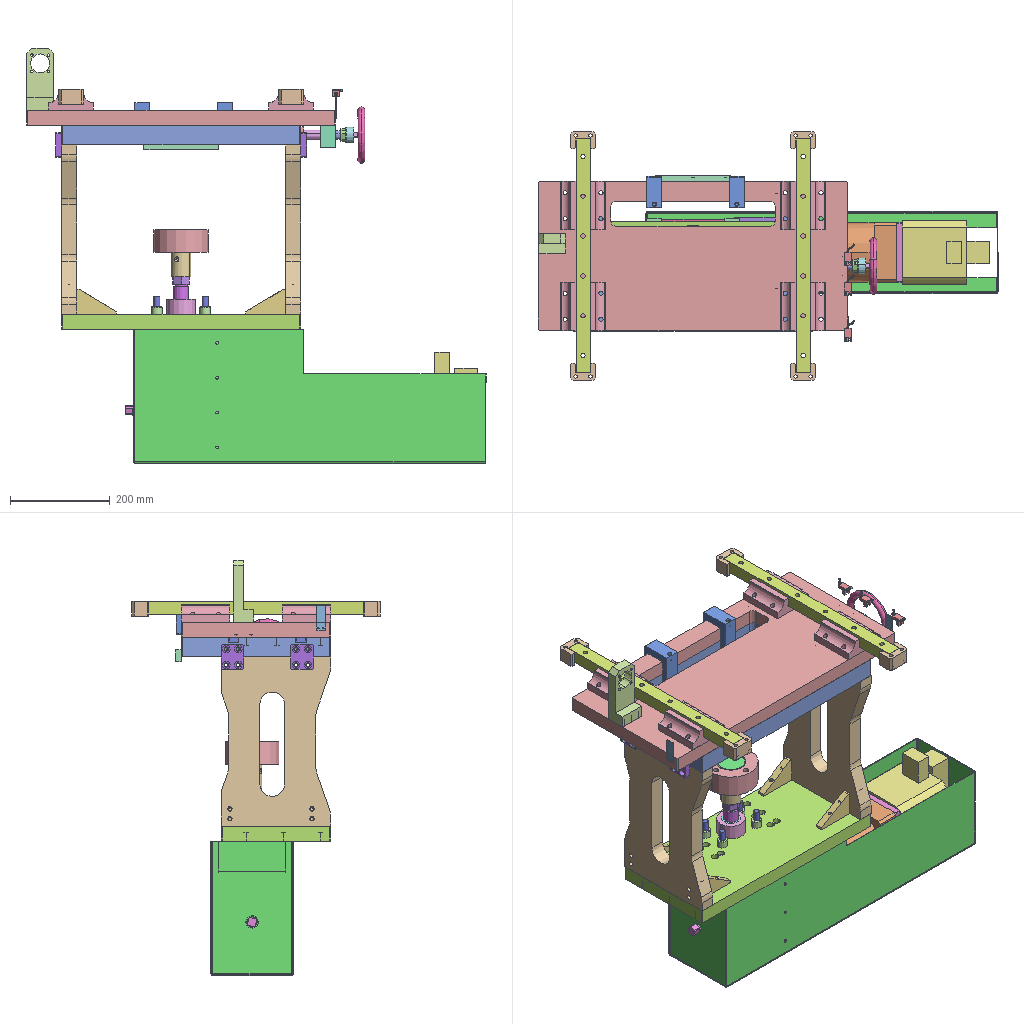Assembly | SolidWorks | 53 different items | 86 placed | box 924 x 500 x 834 mm
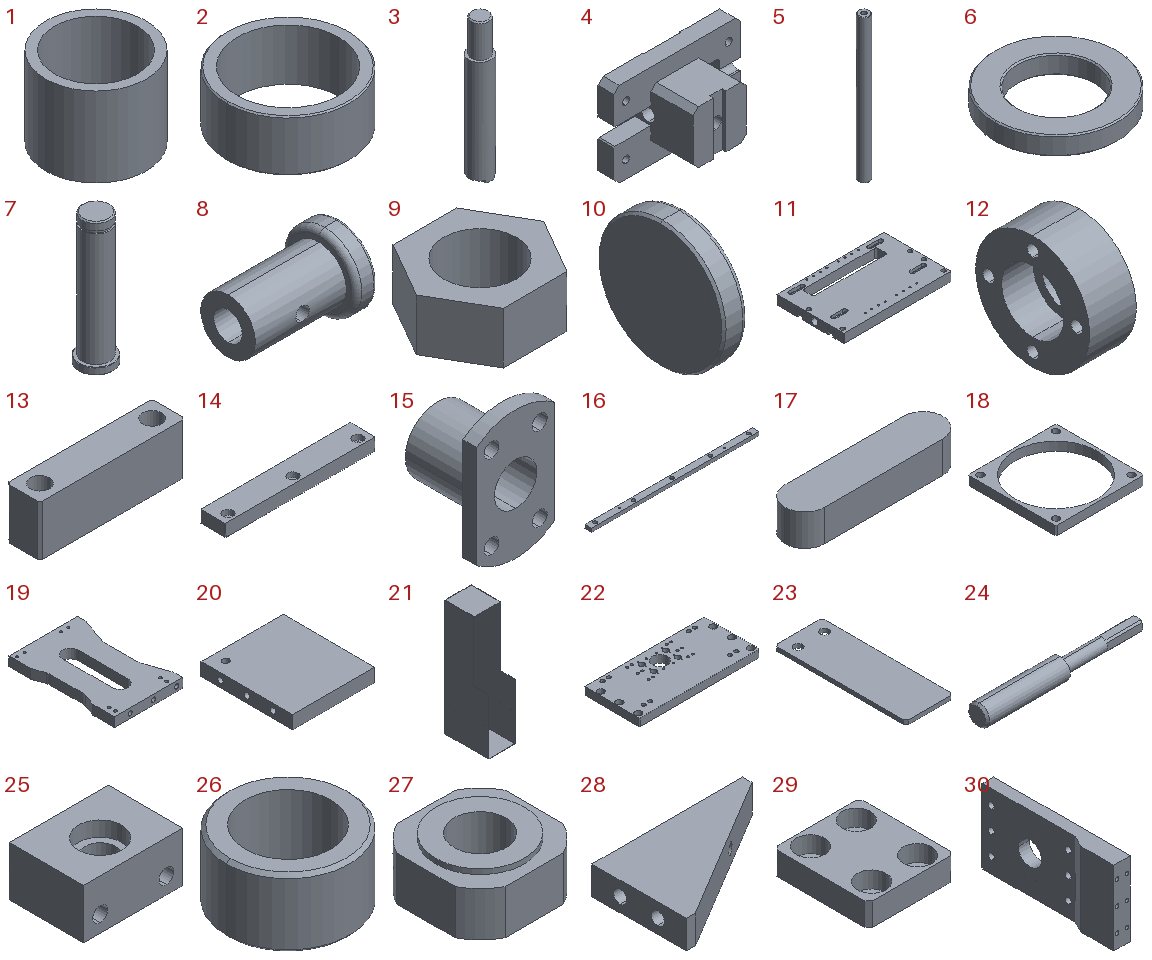Parts list (item | quantity | size | volume | features):
1 | x1 | 48 x 48 x 38 mm | 22197 mm3 | features Extrusion 1
2 | x1 | 48 x 48 x 20 mm | 11645 mm3 | features Chamfer 1, Extrusion 1
3 | x1 | 30 x 30 x 188 mm | 118848 mm3 | features ICE 2, Chamfer 1, Extrusion 1, HoleWzd 1
4 | x1 | 120 x 55 x 80 mm | 190025 mm3 | features ICE 7, Chamfer 2, HoleWzd 2, Extrusion 1
5 | x4 | 12 x 12 x 160 mm | 17782 mm3 | features Chamfer 1, Extrusion 1, HoleWzd 1
6 | x4 | 20 x 20 x 3 mm | 570.238 mm3 | features Chamfer 1, Extrusion 1
7 | x1 | 15 x 15 x 57.5 mm | 6667 mm3 | features Chamfer 2, Extrusion 1, ICE 1, RefAxis 1, RevCut 1
8 | x1 | 82 x 55 x 55 mm | 93090 mm3 | features Fillet 2, HoleWzd 1, ICE 1, Revolution 1
9 | x1 | 36.95 x 32 x 15 mm | 8107 mm3 | features Extrusion 1, HoleWzd 1
10 | x1 | 16.494 x 58 x 58 mm | 35001 mm3 | features Chamfer 1, Fillet 1, Revolution 1
11 | x1 | 480 x 300 x 40 mm | 4575691 mm3 | features HoleWzd 6, ICE 6, Chamfer 1, Extrusion 1, MirrorPattern 1
12 | x1 | 45 x 110 x 110 mm | 290495 mm3 | features HoleWzd 1, Revolution 1
13 | x1 | 26 x 6 x 9 mm | 1236 mm3 | features Chamfer 1, Extrusion 1, HoleWzd 1
14 | x1 | 150 x 25 x 12 mm | 43317 mm3 | features Chamfer 1, Extrusion 1, HoleWzd 1
15 | x1 | 34 x 34 x 56 mm | 17982 mm3 | features HoleWzd 2, ICE 1, Revolution 1
16 | x2 | 480 x 20 x 10 mm | 92979 mm3 | features HoleWzd 2, Chamfer 1, Extrusion 1
17 | x1 | 40 x 10 x 8 mm | 3028 mm3 | features Extrusion 1
18 | x1 | 120 x 120 x 12 mm | 51426 mm3 | features Chamfer 1, CirPattern 1, Extrusion 1, HoleWzd 1, ICE 1
19 | x2 | 220 x 340 x 30 mm | 1630627 mm3 | features HoleWzd 4, Cut 1, Extrusion 1
20 | x2 | 125 x 140 x 20 mm | 339828 mm3 | features HoleWzd 2, Extrusion 1, ICE 1
21 | x1 | 165 x 270 x 708 mm | 725999 mm3 | features EdgeFlange 2, ICE 2, Cut 1, FlatPattern 1, SMBaseFlange 1, SheetMetal 1
22 | x1 | 480 x 220 x 30 mm | 2905739 mm3 | features HoleWzd 5, Chamfer 1, Cut 1, Extrusion 1, ICE 1, MirrorPattern 1
23 | x2 | 18 x 50 x 1.5 mm | 1323 mm3 | features Chamfer 1, Extrusion 1, HoleWzd 1
24 | x1 | 155 x 20 x 20 mm | 32861 mm3 | features Chamfer 2, ICE 1, Revolution 1
25 | x1 | 60 x 45 x 30 mm | 60481 mm3 | features ICE 2, Extrusion 1, HoleWzd 1
26 | x1 | 18 x 18 x 10 mm | 1304 mm3 | features Chamfer 1, Extrusion 1
27 | x1 | 22 x 22 x 10 mm | 3311 mm3 | features HoleWzd 2, 3DProfileFeature 1, Extrusion 1, ICE 1
28 | x4 | 80 x 50 x 15 mm | 31407 mm3 | features HoleWzd 2, Extrusion 1
29 | x4 | 45 x 50 x 12 mm | 19960 mm3 | features Chamfer 1, Extrusion 1, HoleWzd 1
30 | x2 | 30 x 250 x 135 mm | 713772 mm3 | features HoleWzd 4, Chamfer 1, Extrusion 1, ICE 1
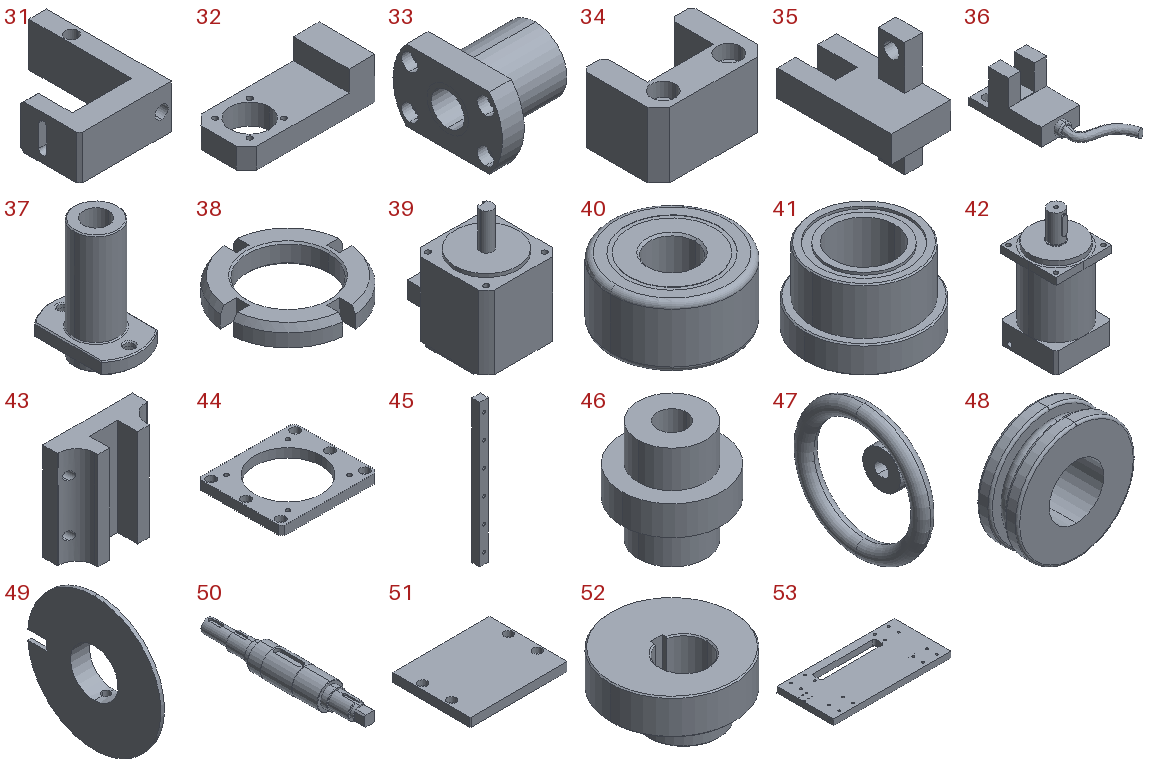31 | x2 | 62.5 x 85 x 30 mm | 56190 mm3 | features ICE 4, HoleWzd 2, Chamfer 1, Extrusion 1
32 | x1 | 124 x 54 x 40 mm | 132841 mm3 | features HoleWzd 2, ICE 2, Chamfer 1, CirPattern 1, Extrusion 1
33 | x1 | 80 x 100 x 65 mm | 212969 mm3 | features ICE 3, HoleWzd 1, Revolution 1
34 | x4 | 50 x 35 x 30 mm | 30679 mm3 | features Chamfer 2, Extrusion 1, HoleWzd 1
35 | x1 | 13.5 x 26 x 26 mm | 2243 mm3 | features Extrusion 1, ICE 1
36 | x3 | 20.544 x 42.48 x 15.5 mm | 2497 mm3 | features ICE 5, 3DProfileFeature 2, Extrusion 1, Fillet 1, Sweep 1
37 | x4 | 27 x 42 x 57 mm | 17013 mm3 | features ICE 4, Chamfer 2, Extrusion 1, HoleWzd 1
38 | x2 | 37.789 x 37.789 x 6 mm | 3246 mm3 | features Chamfer 2, CirPattern 1, Extrusion 1, ICE 1
39 | x1 | 130 x 181 x 245 mm | 2453559 mm3 | features ICE 7, CirPattern 1, Extrusion 1, HoleWzd 1
40 | x1 | 32 x 32 x 16 mm | 10946 mm3 | features ICE 2, Chamfer 1, Extrusion 1, Fillet 1
41 | x2 | 48.2 x 48.2 x 30 mm | 28928 mm3 | features ICE 3, Chamfer 1, Extrusion 1
42 | x1 | 120 x 120 x 255.5 mm | 2340671 mm3 | features Boss 5, ICE 3, CirPattern 2, HoleWzd 2, Chamfer 1, Cut 1, Extrusion 1
43 | x4 | 90 x 36 x 97.4 mm | 192306 mm3 | features Extrusion 1, HoleWzd 1
44 | x1 | 160 x 140 x 15 mm | 176085 mm3 | features HoleWzd 2, CirPattern 1, Extrusion 1, MirrorPattern 1
45 | x2 | 28 x 26 x 470 mm | 326128 mm3 | features Extrusion 1, HoleWzd 1, LPattern 1
46 | x1 | 68 x 68 x 70 mm | 136716 mm3 | features ICE 3, Extrusion 1, MirrorPattern 1
47 | x1 | 39 x 114 x 114 mm | 60150 mm3 | features ICE 2, Chamfer 1, Sweep 1
48 | x2 | 26 x 9 x 26 mm | 3329 mm3 | features Fillet 1, Revolution 1
49 | x1 | 8 x 55.928 x 56 mm | 5685 mm3 | features 3DProfileFeature 1, HoleWzd 1, ICE 1, Revolution 1
50 | x1 | 40 x 245 x 40 mm | 186940 mm3 | features Boss 7, Chamfer 3, ICE 3, Cut 2, Extrusion 1
51 | x1 | 168 x 135 x 15 mm | 332281 mm3 | features Chamfer 1, Extrusion 1, HoleWzd 1
52 | x1 | 105 x 105 x 48 mm | 248122 mm3 | features Boss 1, Chamfer 1, Cut 1, Extrusion 1
53 | x1 | 620 x 300 x 30 mm | 4982142 mm3 | features HoleWzd 9, Chamfer 1, Extrusion 1, ICE 1, LPattern 1, MirrorPattern 1
Mates (type | each side: item.copy, entity, surface, feature):
Coincident | 53.1 face plane Boss-Extrude1 | 11.1 face plane Boss-Extrude1 | 2 times
Width | 53.1 face plane Boss-Extrude1 | 53.1 face plane Boss-Extrude1 | 11.1 face plane Boss-Extrude1 | 11.1 face plane Boss-Extrude1
Concentric | 22.1 face cylinder Cut-Extrude1 | 33.1 face cylinder Revolve1
Parallel | 22.1 face plane Boss-Extrude1 | 33.1 face plane Cut-Extrude1
Coincident | 22.1 face plane Boss-Extrude1 | 33.1 face plane Revolve1
Coincident | 22.1 plane | 3.1 plane
Concentric | 3.1 face cylinder M10 Tapped Hole1 | 4.1 face cylinder CBORE for M10 Hex Socket Head Cap Screw1
Coincident | 3.1 face plane Boss-Extrude3 | 4.1 face plane Cut-Extrude5
Coincident | 3.1 face plane Boss-Extrude1 | 4.1 face plane Boss-Extrude2
Concentric | 4.1 face cylinder Cut-Extrude4 | 40.1 face cylinder Cut-Extrude1
Width | 4.1 face plane Cut-Extrude2 | 4.1 face plane Cut-Extrude2 | 40.1 face plane Boss-Extrude1 | 40.1 face plane Boss-Extrude1
Concentric | 4.1 face cylinder CBORE for M6 Hex Socket Head Cap Screw1 | 5.1 face cylinder Boss-Extrude1
Coincident | 4.1 face plane Boss-Extrude1 | 5.1 face plane Boss-Extrude1
Concentric | 4.1 face cylinder CBORE for M6 Hex Socket Head Cap Screw1 | 5.2 face cylinder Boss-Extrude1
Coincident | 4.1 face plane Boss-Extrude1 | 5.2 face plane Boss-Extrude1
Concentric | 4.1 face cylinder CBORE for M6 Hex Socket Head Cap Screw1 | 5.3 face cylinder Boss-Extrude1
Coincident | 4.1 face plane Boss-Extrude1 | 5.3 face plane Boss-Extrude1
Coincident | 4.1 face plane Boss-Extrude1 | 5.4 face plane Boss-Extrude1
Concentric | 4.1 face cylinder CBORE for M6 Hex Socket Head Cap Screw1 | 5.4 face cylinder Boss-Extrude1
Concentric | 22.1 face cylinder Cut-Extrude2 | 37.1 face cylinder Boss-Extrude3
Coincident | 22.1 face plane Boss-Extrude1 | 37.1 face plane Boss-Extrude2
Concentric | 5.3 face cylinder Boss-Extrude1 | 37.2 face cylinder Cut-Extrude1
Concentric | 22.1 face cylinder Mirror1 | 37.2 face cylinder CBORE for M4 Hex Socket Head Cap Screw1
Coincident | 22.1 face plane Boss-Extrude1 | 37.2 face plane Boss-Extrude2
Concentric | 5.1 face cylinder Boss-Extrude1 | 37.3 face cylinder Boss-Extrude3
Concentric | 22.1 face cylinder M4 Tapped Hole1 | 37.3 face cylinder CBORE for M4 Hex Socket Head Cap Screw1
Coincident | 22.1 face plane Boss-Extrude1 | 37.3 face plane Boss-Extrude2
Concentric | 5.4 face cylinder Boss-Extrude1 | 37.4 face cylinder Boss-Extrude3
Concentric | 22.1 face cylinder Mirror1 | 37.4 face cylinder CBORE for M4 Hex Socket Head Cap Screw1
Coincident | 22.1 face plane Boss-Extrude1 | 37.4 face plane Boss-Extrude2
Concentric | 5.2 face cylinder Boss-Extrude1 | 6.1 edge
Coincident | 37.1 face plane Boss-Extrude1 | 6.1 face plane Boss-Extrude1
Concentric | 5.1 face cylinder Boss-Extrude1 | 6.2 face cylinder Boss-Extrude1
Coincident | 37.3 face plane Boss-Extrude1 | 6.2 face plane Boss-Extrude1
Concentric | 5.4 face cylinder Boss-Extrude1 | 6.3 face cylinder Boss-Extrude1
Coincident | 37.4 face plane Boss-Extrude1 | 6.3 face plane Boss-Extrude1
Coincident | 6.3 face plane Boss-Extrude1 | 6.4 face plane Boss-Extrude1
Concentric | 5.3 face cylinder Boss-Extrude1 | 6.4 face cylinder Boss-Extrude1
Concentric | 4.1 face cylinder Cut-Extrude4 | 7.1 face cylinder Boss-Extrude2
Coincident | 4.1 face plane Boss-Extrude2 | 7.1 face plane Boss-Extrude1
DistanceDim | 9.1 face plane Boss-Extrude1 | 3.1 face plane Boss-Extrude1
Coincident | 8.1 face plane Revolve1 | 9.1 face plane Boss-Extrude1
Concentric | 8.1 face cylinder Revolve1 | 10.1 face cylinder Revolve1
Tangent | 8.1 face sphere Revolve1 | 10.1 face sphere Revolve1
Coincident | 10.1 face plane Revolve1 | 12.1 face plane Revolve1
Concentric | 3.1 face cylinder Boss-Extrude2 | 9.1 face cylinder M24 Tapped Hole1
Concentric | 3.1 face cylinder Boss-Extrude1 | 8.1 face cylinder Revolve1
Concentric | 35.1 face cylinder Boss-Extrude2 | 13.1 face cylinder M3 Clearance Hole1 | 2 times
Coincident | 35.1 face plane Boss-Extrude1 | 13.1 face plane Boss-Extrude1
Parallel | 49.1 plane | 51.1 face plane Boss-Extrude1
Coincident | 49.1 plane | 35.1 plane
Concentric | 44.1 face cylinder Boss-Extrude1 | 42.1 face cylinder Extrude2
Coincident | 44.1 face plane Boss-Extrude1 | 42.1 face plane Extrude2
Concentric | 42.1 face cylinder Cut-Extrude2 | 39.1 face cylinder Boss-Extrude3
Concentric | 42.1 face cylinder CirPattern1 | 39.1 face cylinder CirPattern1
DistanceDim | 42.1 face plane Extrude1 | 39.1 face plane Boss-Extrude1
Coincident | 11.1 face plane Boss-Extrude1 | 14.1 face plane Boss-Extrude1
Concentric | 11.1 face cylinder M5 Tapped Hole1 | 14.1 face cylinder CBORE for M5 Hex Socket Head Cap Screw1 | 2 times
Coincident | 53.1 face plane Boss-Extrude1 | 16.1 face plane Boss-Extrude1
Width | 16.1 face plane Boss-Extrude1 | 16.1 face plane Boss-Extrude1 | 11.1 face plane Boss-Extrude1 | 11.1 face plane Boss-Extrude1
Coincident | 53.1 face plane Boss-Extrude1 | 16.2 face plane Boss-Extrude1
Coincident | 16.1 face plane Boss-Extrude1 | 16.2 face plane Boss-Extrude1
Concentric | 39.1 face cylinder Boss-Extrude2 | 18.1 face cylinder Cut-Extrude1
Parallel | 42.1 face plane Extrude1 | 18.1 face plane Boss-Extrude1
Coincident | 42.1 face plane Extrude1 | 18.1 face plane Boss-Extrude1
Parallel | 44.1 face plane Boss-Extrude1 | 42.1 face plane Boss-Extrude1
Coincident | 11.1 face plane Cut-Extrude2 | 16.1 face plane Boss-Extrude1
Coincident | 11.1 face plane Cut-Extrude2 | 16.2 face plane Boss-Extrude1
Parallel | 11.1 face plane Boss-Extrude1 | 15.1 face plane Cut-Extrude1
Coincident | 38.1 face plane Boss-Extrude1 | 41.1 face plane Boss-Extrude2
Coincident | 41.2 face plane Boss-Extrude2 | 38.2 face plane Boss-Extrude1
Coincident | 22.1 face plane Boss-Extrude1 | 19.1 face plane Boss-Extrude1 | 3 times
Coincident | 22.1 face plane Boss-Extrude1 | 19.2 face plane Boss-Extrude1 | 2 times
Coincident | 19.1 face plane Boss-Extrude1 | 19.2 face plane Boss-Extrude1
Coincident | 11.1 face plane Boss-Extrude1 | 19.1 face plane Boss-Extrude1
Width | 19.1 face plane Boss-Extrude1 | 19.2 face plane Boss-Extrude1 | 11.1 face plane Boss-Extrude1 | 11.1 face plane Boss-Extrude1
Coincident | 11.1 face plane Boss-Extrude1 | 19.2 face plane Boss-Extrude1
Coincident | 44.1 face plane Boss-Extrude1 | 20.1 face plane Boss-Extrude1 | 3 times
Concentric | 42.1 face cylinder Extrude5 | 46.1 face cylinder Mirror1
Parallel | 51.1 face plane Boss-Extrude1 | 20.1 face plane Boss-Extrude1
Coincident | 44.1 face plane Boss-Extrude1 | 20.2 face plane Boss-Extrude1 | 2 times
Coincident | 20.1 face plane Boss-Extrude1 | 20.2 face plane Boss-Extrude1
Coincident | 43.1 face plane Boss-Extrude1 | 43.2 face plane Boss-Extrude1
Coincident | 43.1 face plane Boss-Extrude1 | 43.3 face plane Boss-Extrude1
Coincident | 43.4 face plane Boss-Extrude1 | 43.1 face plane Boss-Extrude1
Concentric | 53.1 face cylinder Hole size per socket head cap screw type2 | 43.3 face cylinder M10 Tapped Hole1 | 2 times
Concentric | 53.1 edge | 43.1 face cylinder M10 Tapped Hole1
Concentric | 53.1 face cylinder Hole size per socket head cap screw type2 | 43.1 face cylinder M10 Tapped Hole1
Concentric | 53.1 edge | 43.2 face cylinder M10 Tapped Hole1
Concentric | 53.1 face cylinder Hole size per socket head cap screw type2 | 43.2 face cylinder M10 Tapped Hole1
Concentric | 53.1 face cylinder Hole size per socket head cap screw type2 | 43.4 face cylinder M10 Tapped Hole1 | 2 times
Coincident | 53.1 face plane Boss-Extrude1 | 43.4 face plane Boss-Extrude1
Coincident | 53.1 face plane Boss-Extrude1 | 23.1 face plane Boss-Extrude1
Concentric | 53.1 edge | 23.1 face cylinder Ø3.2 (3.2) Diameter Hole1
Concentric | 53.1 face cylinder M3 Tapped Hole2 | 23.1 face cylinder Ø3.2 (3.2) Diameter Hole1
Coincident | 53.1 face plane Boss-Extrude1 | 23.2 face plane Boss-Extrude1
Concentric | 53.1 face cylinder Mirror2 | 23.2 face cylinder Ø3.2 (3.2) Diameter Hole1 | 2 times
Coincident | 53.1 face plane Boss-Extrude1 | 32.1 face plane Boss-Extrude1
Concentric | 53.1 face cylinder Hole size per socket head cap screw type0 | 32.1 face cylinder M6 Tapped Hole2 | 2 times
Coincident | 43.1 face plane Boss-Extrude1 | 45.1 face plane Boss-Extrude1
Width | 43.2 face plane Boss-Extrude1 | 43.2 face plane Boss-Extrude1 | 45.2 face plane Boss-Extrude1 | 45.2 face plane Boss-Extrude1
Coincident | 45.1 face plane Boss-Extrude1 | 45.2 face plane Boss-Extrude1 | 2 times
Concentric | 24.1 face cylinder Revolve1 | 48.1 face cylinder Revolve1
Coincident | 24.1 face plane Revolve1 | 48.1 face plane Revolve1
Concentric | 24.1 face cylinder Revolve1 | 48.2 face cylinder Revolve1
Concentric | 24.1 face cylinder Revolve1 | 26.1 face cylinder Boss-Extrude1
Concentric | 24.1 face cylinder Revolve1 | 27.1 face cylinder M12x1.5 Tapped Hole1
Coincident | 24.1 face plane Cut-Extrude1 | 47.1 face plane Cut-Extrude1
Concentric | 25.1 face cylinder Extrude1 | 48.1 face cylinder Revolve1
Coincident | 25.1 face plane Boss-Extrude1 | 48.1 face plane Revolve1
Coincident | 25.1 face plane Extrude2 | 48.2 face plane Revolve1
Coincident | 48.2 face plane Revolve1 | 26.1 face plane Boss-Extrude1
Coincident | 26.1 face plane Boss-Extrude1 | 27.1 face plane Extrude1
Concentric | 26.1 face cylinder Boss-Extrude1 | 47.1 face cylinder Boss-Extrude1
Concentric | 15.1 edge | 24.1 face cylinder Revolve1
Coincident | 27.1 face plane Extrude1 | 47.1 face plane Boss-Extrude1
Width | 43.4 face plane Boss-Extrude1 | 43.4 face plane Boss-Extrude1 | 45.1 face plane Boss-Extrude1 | 45.1 face plane Boss-Extrude1
Concentric | 8.1 face cylinder Revolve1 | 12.1 face cylinder Revolve1
Concentric | 11.1 face cylinder Cut-Extrude8 | 15.1 face cylinder Revolve1
Coincident | 11.1 face plane Boss-Extrude1 | 15.1 face plane Revolve1
Parallel | 53.1 face plane Boss-Extrude1 | 15.1 face plane Cut-Extrude1
Coincident | 53.1 face plane Boss-Extrude1 | 25.1 face plane Boss-Extrude1 | 2 times
DistanceDim | 53.1 face plane Boss-Extrude1 | 45.1 face plane Boss-Extrude1
Coincident | 19.1 face plane Boss-Extrude1 | 28.1 face plane Boss-Extrude1
Coincident | 22.1 face plane Boss-Extrude1 | 28.1 face plane Boss-Extrude1
Coincident | 22.1 face plane Boss-Extrude1 | 28.2 face plane Boss-Extrude1
Coincident | 19.2 face plane Boss-Extrude1 | 28.2 face plane Boss-Extrude1
Coincident | 19.1 face plane Boss-Extrude1 | 28.3 face plane Boss-Extrude1
Coincident | 22.1 face plane Boss-Extrude1 | 28.4 face plane Boss-Extrude1
Coincident | 19.2 face plane Boss-Extrude1 | 28.4 face plane Boss-Extrude1
Coincident | 28.3 face plane Boss-Extrude1 | 28.4 face plane Boss-Extrude1
DistanceDim | 28.4 face plane Boss-Extrude1 | 22.1 face plane Boss-Extrude1
Coincident | 19.1 face plane Boss-Extrude1 | 29.1 face plane Boss-Extrude1
DistanceDim | 29.1 face plane Boss-Extrude1 | 11.1 face plane Boss-Extrude1 | 2 times
Coincident | 29.1 face plane Boss-Extrude1 | 29.2 face plane Boss-Extrude1 | 2 times
Coincident | 19.1 face plane Cut-Extrude1 | 29.2 face plane Boss-Extrude1
Coincident | 28.1 face plane Boss-Extrude1 | 28.2 face plane Boss-Extrude1
DistanceDim | 28.1 face plane Boss-Extrude1 | 22.1 face plane Boss-Extrude1
Coincident | 22.1 face plane Boss-Extrude1 | 30.1 face plane Boss-Extrude1
Concentric | 41.2 face cylinder Boss-Extrude2 | 30.1 face cylinder Cut-Extrude1
Concentric | 22.1 face cylinder Hole Size Based On Hex Socket Head Cap Screw Type2 | 30.1 face cylinder M8 Tapped Hole1 | 2 times
Coincident | 20.1 face plane Boss-Extrude1 | 30.2 face plane Boss-Extrude1
Coincident | 51.1 face plane Boss-Extrude1 | 30.2 face plane Boss-Extrude1 | 2 times
Coincident | 51.1 face plane Boss-Extrude1 | 30.1 face plane Boss-Extrude1 | 3 times
Coincident | 30.1 face plane Boss-Extrude1 | 30.2 face plane Boss-Extrude1
Coincident | 41.2 face plane Boss-Extrude1 | 30.1 face plane Boss-Extrude1
Coincident | 45.2 face plane Boss-Extrude1 | 36.1 face plane Boss-Extrude1
Coincident | 36.1 face plane Boss-Extrude1 | 36.2 face plane Boss-Extrude1 | 2 times
Coincident | 36.2 face plane Boss-Extrude1 | 36.3 face plane Boss-Extrude1 | 2 times
Width | 36.2 face plane Cut-Extrude3 | 36.2 face plane Cut-Extrude3 | 23.2 face plane Boss-Extrude1 | 23.2 face plane Boss-Extrude1
Coincident | 53.1 face plane Boss-Extrude1 | 31.1 face plane Boss-Extrude1 | 2 times
Coincident | 31.1 face plane Boss-Extrude1 | 31.2 face plane Boss-Extrude1 | 2 times
Width | 21.1 face plane Base-Flange1 | 21.1 face plane Base-Flange1 | 20.1 face plane Boss-Extrude1 | 20.1 face plane Boss-Extrude1
DistanceDim | 50.1 face plane Boss-Extrude1 | 30.1 face plane Boss-Extrude1
Concentric | 41.2 face cylinder Boss-Extrude2 | 50.1 face cylinder Extrude6
Concentric | 38.2 face cylinder Boss-Extrude1 | 50.1 face cylinder Extrude6
Concentric | 41.1 face cylinder Boss-Extrude2 | 50.1 face cylinder Extrude2
Coincident | 41.1 face plane Boss-Extrude1 | 30.2 face plane Boss-Extrude1
Coincident | 17.1 face plane Boss-Extrude1 | 50.1 face plane Cut-Extrude1
Concentric | 17.1 face cylinder Boss-Extrude1 | 50.1 face cylinder Cut-Extrude1
Concentric | 50.1 face cylinder Extrude1 | 52.1 face cylinder Extrude2
Coincident | 1.1 face plane Boss-Extrude1 | 41.2 face plane Boss-Extrude1
Concentric | 1.1 face cylinder Boss-Extrude1 | 50.1 face cylinder Extrude1
Coincident | 1.1 face plane Boss-Extrude1 | 52.1 face plane Extrude1
Coincident | 2.1 face plane Boss-Extrude1 | 41.1 face plane Boss-Extrude1
Concentric | 2.1 face cylinder Boss-Extrude1 | 50.1 face cylinder Extrude2
Tangent | 40.1 face cylinder Boss-Extrude1 | 52.1 face cylinder Extrude1
Coincident | 50.1 plane | 52.1 plane
Concentric | 49.1 face cylinder Revolve1 | 50.1 face cylinder Extrude7
Concentric | 38.1 face cylinder Boss-Extrude1 | 50.1 face cylinder Extrude4
Coincident | 13.1 face plane Boss-Extrude1 | 30.2 face plane Boss-Extrude1
Concentric | 46.1 face cylinder Boss-Extrude2 | 50.1 face cylinder Extrude7
Coincident | 46.1 face plane Boss-Extrude1 | 50.1 face plane Extrude7
Width | 49.1 face plane Revolve1 | 49.1 face plane Revolve1 | 35.1 face plane Boss-Extrude1 | 35.1 face plane Boss-Extrude1
Concentric | 35.1 face cylinder Boss-Extrude2 | 30.2 face cylinder M3 Tapped Hole1
Coincident | 21.1 face plane Edge-Flange1 | 30.1 face plane Boss-Extrude1
Coincident | 22.1 face plane Boss-Extrude1 | 21.1 face plane Edge-Flange1
Coincident | 45.2 face plane Boss-Extrude1 | 34.1 face plane Boss-Extrude1 | 2 times
Width | 34.1 face plane Boss-Extrude1 | 34.1 face plane Boss-Extrude1 | 45.2 face plane Boss-Extrude1 | 45.2 face plane Boss-Extrude1
Coincident | 34.1 face plane Boss-Extrude1 | 34.2 face plane Boss-Extrude1 | 2 times
Width | 34.2 face plane Boss-Extrude1 | 34.2 face plane Boss-Extrude1 | 45.1 face plane Boss-Extrude1 | 45.1 face plane Boss-Extrude1
Coincident | 45.2 face plane Boss-Extrude1 | 34.3 face plane Boss-Extrude1
Coincident | 34.1 face plane Boss-Extrude1 | 34.3 face plane Boss-Extrude1
Width | 34.3 face plane Boss-Extrude1 | 34.3 face plane Boss-Extrude1 | 45.2 face plane Boss-Extrude1 | 45.2 face plane Boss-Extrude1
Coincident | 34.3 face plane Boss-Extrude1 | 34.4 face plane Boss-Extrude1 | 2 times
Width | 34.4 face plane Boss-Extrude1 | 34.4 face plane Boss-Extrude1 | 45.1 face plane Boss-Extrude1 | 45.1 face plane Boss-Extrude1